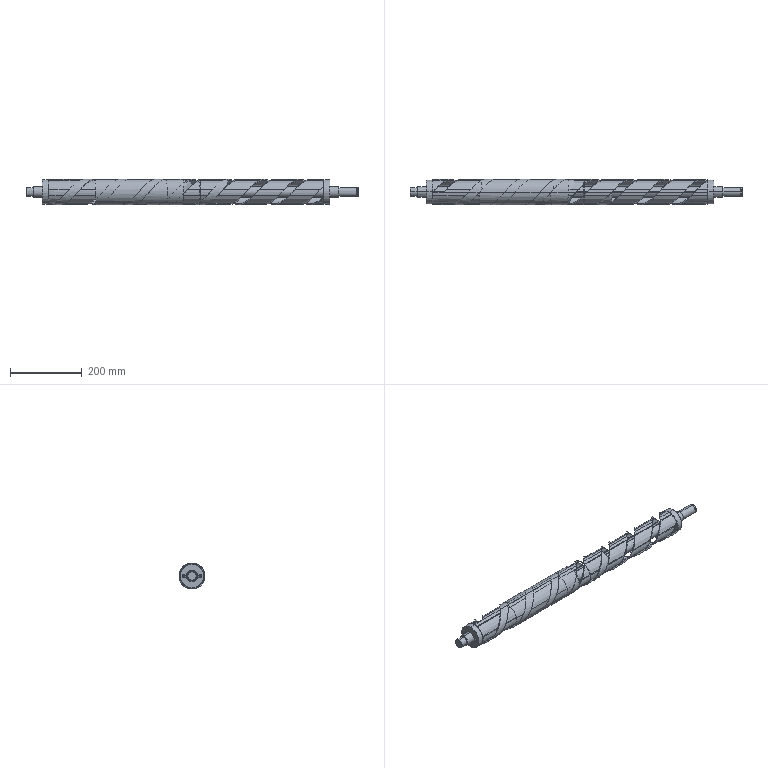Part | SolidWorks | features LayoutProfileFeature 1 | 5 solids | 262 faces | box 926 x 81.066 x 72.005 mm | volume 3183624 mm3 | cylinder 124 | plane 99 | cone 20 | spline 19 | commonest cylinder face diameters 70 x42 65 x34 72 x14 8 x6 25 x6 7 x4